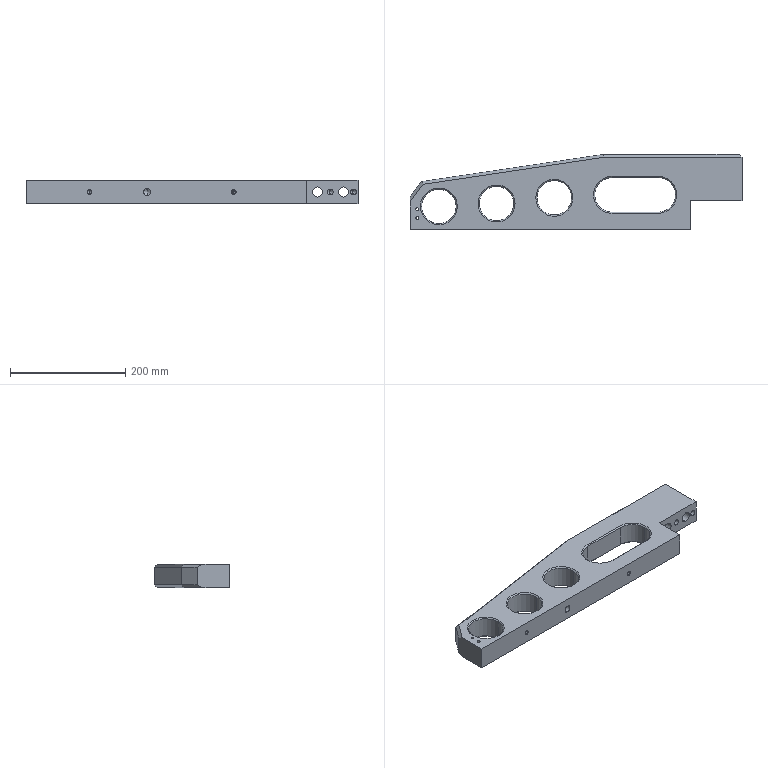Part | STEP file | reinforcing fixing bracket | 1 solid | 90 faces | box 575 x 130 x 40 mm | volume 1733359 mm3 | cone 34 | cylinder 31 | plane 25 | commonest cylinder face diameters 60 x9 5 x4 6.8 x4 10 x4 17.5 x4 26 x4